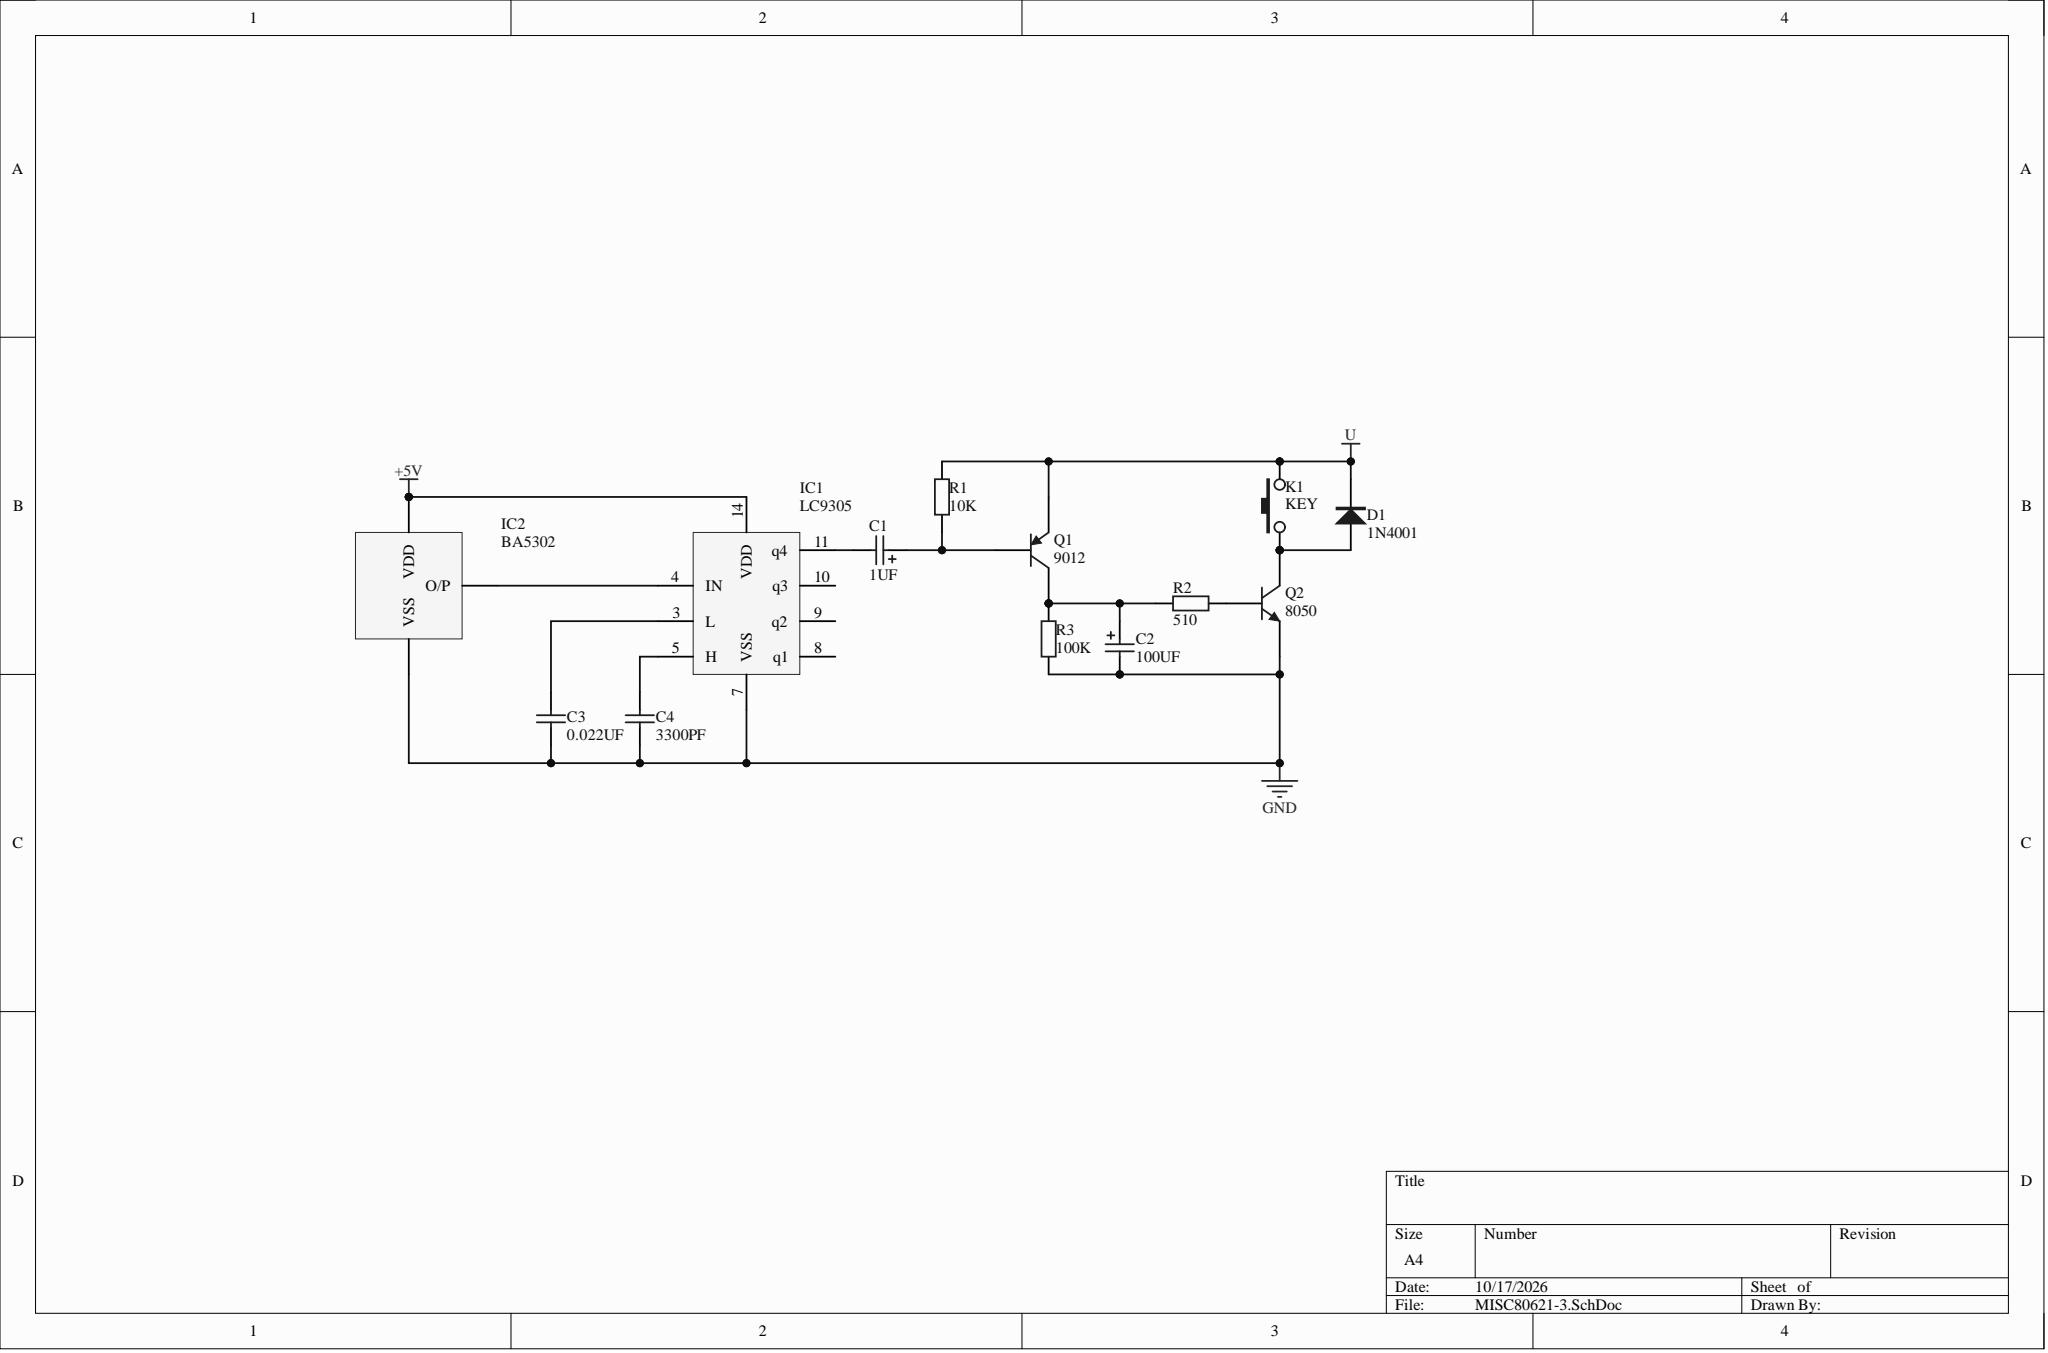Circuit board | Altium Designer | 13 parts | 11 nets
Bill of materials:
Comment,Description,Designator,Footprint,LibRef,Quantity
"1UF","Polarized Capacitor (Axial)","C1","POLAR0.8","Cap Pol2","1"
"100UF","Polarized Capacitor (Axial)","C2","POLAR0.8","Cap Pol2","1"
"0.022UF","Capacitor","C3","RAD-0.3","Cap","1"
"3300PF","Capacitor","C4","RAD-0.3","Cap","1"
"1N4001","Rectifier diode","D1","DO-41","1N4007","1"
"LC9305","","IC1","DIP14","LC9305","1"
"BA5302","","IC2","HDR1X3","BA5302","1"
"KEY","","K1","DIP-3X6X4.3","KEY","1"
"9012","PNP General Purpose Amplifier","Q1","TO-92A","2N3906","1"
"8050","NPN General Purpose Amplifier","Q2","TO-92A","2N3904","1"
"10K","Resistor","R1","AXIAL-0.4","Res2","1"
"510","Resistor","R2","AXIAL-0.4","Res2","1"
"100K","Resistor","R3","AXIAL-0.4","Res2","1"
Netlist (Protel format):
[
C1
POLAR0.8
1UF



]
[
C2
POLAR0.8
100UF



]
[
C3
RAD-0.3
0.022UF



]
[
C4
RAD-0.3
3300PF



]
[
D1
DO-41
1N4001



]
[
IC1
DIP14
LC9305



]
[
IC2
HDR1X3
BA5302



]
[
K1
DIP-3X6X4.3
KEY



]
[
Q1
TO-92A
9012



]
[
Q2
TO-92A
8050



]
[
R1
AXIAL-0.4
10K



]
[
R2
AXIAL-0.4
510



]
[
R3
AXIAL-0.4
100K



]
(
U
D1-2
K1-3
Q1-1
R1-2
)
(
NetQ2_2
Q2-2
R2-1
)
(
NetIC1_4
IC1-4
IC2-2
)
(
NetD1_1
D1-1
K1-1
Q2-3
)
(
NetC4_2
C4-2
IC1-5
)
(
NetC3_2
C3-2
IC1-3
)
(
NetC2_1
C2-1
Q1-3
R2-2
R3-2
)
(
NetC1_2
C1-2
IC1-11
)
(
NetC1_1
C1-1
Q1-2
R1-1
)
(
GND
C2-2
C3-1
C4-1
IC1-7
IC2-3
Q2-1
R3-1
)
(
+5V
IC1-14
IC2-1
)